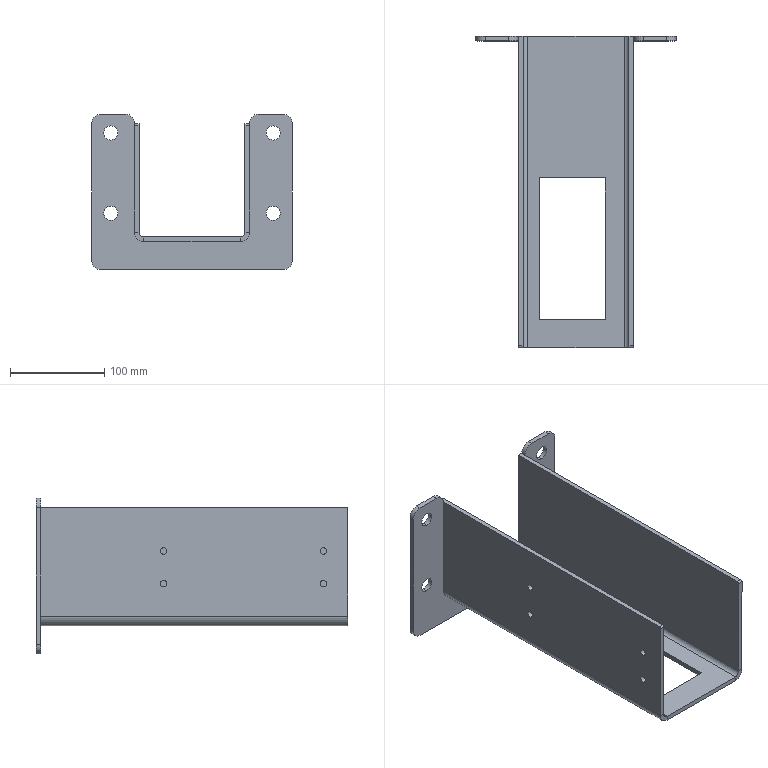Part | SolidWorks | features ICE 3, Fillet 2, EdgeFlange 1, FlatPattern 1, HoleWzd 1, SMBaseFlange 1, SheetMetal 1 | 2 solids | 62 faces | box 212 x 330 x 165 mm | volume 621985 mm3 | plane 32 | cylinder 30 | commonest cylinder face diameters 20 x10 7 x8 15 x8 4 x2 10 x2